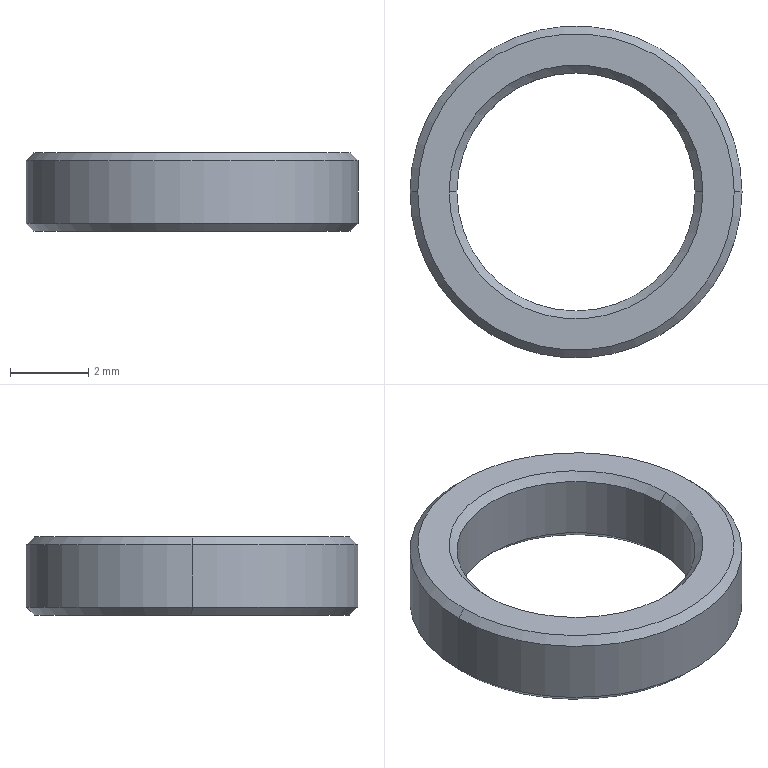Part | NX | features BREP 1 | 1 solid | 14 faces | box 8.5 x 8.5 x 2 mm | volume 53.206 mm3 | cone 8 | cylinder 4 | plane 2 | commonest cylinder face diameters 6.1 x2 8.5 x2
STEP:
#1=CARTESIAN_POINT('',(-3.25,0.,2.));
#2=VERTEX_POINT('',#1);
#3=CARTESIAN_POINT('',(-3.05,0.,1.8));
#4=VERTEX_POINT('',#3);
#5=CARTESIAN_POINT('',(-3.05,0.,1.8));
#6=DIRECTION('',(-0.7071,0.,0.7071));
#7=VECTOR('',#6,1000.);
#8=LINE('',#5,#7);
#9=EDGE_CURVE('',#2,#4,#8,.F.);
#10=ORIENTED_EDGE('',*,*,#9,.T.);
#11=CARTESIAN_POINT('',(3.05,0.,1.8));
#12=VERTEX_POINT('',#11);
#13=CARTESIAN_POINT('',(0.,0.,1.8));
#14=DIRECTION('',(0.,0.,1.));
#15=DIRECTION('',(1.,0.,0.));
#16=AXIS2_PLACEMENT_3D('',#13,#14,#15);
#17=CIRCLE('',#16,3.05);
#18=EDGE_CURVE('',#12,#4,#17,.T.);
#19=ORIENTED_EDGE('',*,*,#18,.F.);
#20=CARTESIAN_POINT('',(3.25,0.,2.));
#21=VERTEX_POINT('',#20);
#22=CARTESIAN_POINT('',(3.05,0.,1.8));
#23=DIRECTION('',(0.7071,0.,0.7071));
#24=VECTOR('',#23,1000.);
#25=LINE('',#22,#24);
#26=EDGE_CURVE('',#21,#12,#25,.F.);
#27=ORIENTED_EDGE('',*,*,#26,.F.);
#28=CARTESIAN_POINT('',(0.,0.,2.));
#29=DIRECTION('',(0.,0.,-1.));
#30=DIRECTION('',(1.,0.,0.));
#31=AXIS2_PLACEMENT_3D('',#28,#29,#30);
#32=CIRCLE('',#31,3.25);
#33=EDGE_CURVE('',#2,#21,#32,.T.);
#34=ORIENTED_EDGE('',*,*,#33,.F.);
#35=EDGE_LOOP('',(#10,#19,#27,#34));
#36=FACE_BOUND('',#35,.T.);
#37=CARTESIAN_POINT('',(0.,0.,1.8));
#38=DIRECTION('',(0.,0.,1.));
#39=DIRECTION('',(1.,0.,0.));
#40=AXIS2_PLACEMENT_3D('',#37,#38,#39);
#41=CONICAL_SURFACE('',#40,3.05,0.7854);
#42=ADVANCED_FACE('',(#36),#41,.F.);
#43=CARTESIAN_POINT('',(4.05,0.,2.));
#44=VERTEX_POINT('',#43);
#45=CARTESIAN_POINT('',(4.25,0.,1.8));
#46=VERTEX_POINT('',#45);
#47=CARTESIAN_POINT('',(4.05,0.,2.));
#48=DIRECTION('',(0.7071,0.,-0.7071));
#49=VECTOR('',#48,1000.);
#50=LINE('',#47,#49);
#51=EDGE_CURVE('',#44,#46,#50,.T.);
#52=ORIENTED_EDGE('',*,*,#51,.F.);
#53=CARTESIAN_POINT('',(-4.05,0.,2.));
#54=VERTEX_POINT('',#53);
#55=CARTESIAN_POINT('',(0.,0.,2.));
#56=DIRECTION('',(0.,0.,1.));
#57=DIRECTION('',(1.,0.,0.));
#58=AXIS2_PLACEMENT_3D('',#55,#56,#57);
#59=CIRCLE('',#58,4.05);
#60=EDGE_CURVE('',#54,#44,#59,.T.);
#61=ORIENTED_EDGE('',*,*,#60,.F.);
#62=CARTESIAN_POINT('',(-4.25,0.,1.8));
#63=VERTEX_POINT('',#62);
#64=CARTESIAN_POINT('',(-4.05,0.,2.));
#65=DIRECTION('',(-0.7071,0.,-0.7071));
#66=VECTOR('',#65,1000.);
#67=LINE('',#64,#66);
#68=EDGE_CURVE('',#54,#63,#67,.T.);
#69=ORIENTED_EDGE('',*,*,#68,.T.);
#70=CARTESIAN_POINT('',(0.,0.,1.8));
#71=DIRECTION('',(0.,0.,-1.));
#72=DIRECTION('',(1.,0.,0.));
#73=AXIS2_PLACEMENT_3D('',#70,#71,#72);
#74=CIRCLE('',#73,4.25);
#75=EDGE_CURVE('',#46,#63,#74,.T.);
#76=ORIENTED_EDGE('',*,*,#75,.F.);
#77=EDGE_LOOP('',(#52,#61,#69,#76));
#78=FACE_BOUND('',#77,.T.);
#79=CARTESIAN_POINT('',(0.,0.,2.));
#80=DIRECTION('',(0.,0.,-1.));
#81=DIRECTION('',(-1.,0.,0.));
#82=AXIS2_PLACEMENT_3D('',#79,#80,#81);
#83=CONICAL_SURFACE('',#82,4.05,0.7854);
#84=ADVANCED_FACE('',(#78),#83,.T.);
#85=CARTESIAN_POINT('',(3.05,0.,0.2));
#86=VERTEX_POINT('',#85);
#87=CARTESIAN_POINT('',(3.25,0.,0.));
#88=VERTEX_POINT('',#87);
#89=CARTESIAN_POINT('',(3.25,0.,0.));
#90=DIRECTION('',(0.7071,0.,-0.7071));
#91=VECTOR('',#90,1000.);
#92=LINE('',#89,#91);
#93=EDGE_CURVE('',#86,#88,#92,.T.);
#94=ORIENTED_EDGE('',*,*,#93,.F.);
#95=CARTESIAN_POINT('',(-3.05,0.,0.2));
#96=VERTEX_POINT('',#95);
#97=CARTESIAN_POINT('',(0.,0.,0.2));
#98=DIRECTION('',(0.,0.,-1.));
#99=DIRECTION('',(1.,0.,0.));
#100=AXIS2_PLACEMENT_3D('',#97,#98,#99);
#101=CIRCLE('',#100,3.05);
#102=EDGE_CURVE('',#96,#86,#101,.T.);
#103=ORIENTED_EDGE('',*,*,#102,.F.);
#104=CARTESIAN_POINT('',(-3.25,0.,0.));
#105=VERTEX_POINT('',#104);
#106=CARTESIAN_POINT('',(-3.25,0.,0.));
#107=DIRECTION('',(-0.7071,0.,-0.7071));
#108=VECTOR('',#107,1000.);
#109=LINE('',#106,#108);
#110=EDGE_CURVE('',#96,#105,#109,.T.);
#111=ORIENTED_EDGE('',*,*,#110,.T.);
#112=CARTESIAN_POINT('',(0.,0.,0.));
#113=DIRECTION('',(0.,0.,1.));
#114=DIRECTION('',(1.,0.,0.));
#115=AXIS2_PLACEMENT_3D('',#112,#113,#114);
#116=CIRCLE('',#115,3.25);
#117=EDGE_CURVE('',#88,#105,#116,.T.);
#118=ORIENTED_EDGE('',*,*,#117,.F.);
#119=EDGE_LOOP('',(#94,#103,#111,#118));
#120=FACE_BOUND('',#119,.T.);
#121=CARTESIAN_POINT('',(0.,0.,0.));
#122=DIRECTION('',(0.,0.,-1.));
#123=DIRECTION('',(-1.,0.,0.));
#124=AXIS2_PLACEMENT_3D('',#121,#122,#123);
#125=CONICAL_SURFACE('',#124,3.25,0.7854);
#126=ADVANCED_FACE('',(#120),#125,.F.);
#127=CARTESIAN_POINT('',(-4.25,0.,0.2));
#128=VERTEX_POINT('',#127);
#129=CARTESIAN_POINT('',(-4.05,0.,0.));
#130=VERTEX_POINT('',#129);
#131=CARTESIAN_POINT('',(-4.25,0.,0.2));
#132=DIRECTION('',(-0.7071,0.,0.7071));
#133=VECTOR('',#132,1000.);
#134=LINE('',#131,#133);
#135=EDGE_CURVE('',#128,#130,#134,.F.);
#136=ORIENTED_EDGE('',*,*,#135,.T.);
#137=CARTESIAN_POINT('',(4.05,0.,0.));
#138=VERTEX_POINT('',#137);
#139=CARTESIAN_POINT('',(0.,0.,0.));
#140=DIRECTION('',(0.,0.,-1.));
#141=DIRECTION('',(1.,0.,0.));
#142=AXIS2_PLACEMENT_3D('',#139,#140,#141);
#143=CIRCLE('',#142,4.05);
#144=EDGE_CURVE('',#138,#130,#143,.T.);
#145=ORIENTED_EDGE('',*,*,#144,.F.);
#146=CARTESIAN_POINT('',(4.25,0.,0.2));
#147=VERTEX_POINT('',#146);
#148=CARTESIAN_POINT('',(4.25,0.,0.2));
#149=DIRECTION('',(0.7071,0.,0.7071));
#150=VECTOR('',#149,1000.);
#151=LINE('',#148,#150);
#152=EDGE_CURVE('',#147,#138,#151,.F.);
#153=ORIENTED_EDGE('',*,*,#152,.F.);
#154=CARTESIAN_POINT('',(0.,0.,0.2));
#155=DIRECTION('',(0.,0.,1.));
#156=DIRECTION('',(1.,0.,0.));
#157=AXIS2_PLACEMENT_3D('',#154,#155,#156);
#158=CIRCLE('',#157,4.25);
#159=EDGE_CURVE('',#128,#147,#158,.T.);
#160=ORIENTED_EDGE('',*,*,#159,.F.);
#161=EDGE_LOOP('',(#136,#145,#153,#160));
#162=FACE_BOUND('',#161,.T.);
#163=CARTESIAN_POINT('',(0.,0.,0.2));
#164=DIRECTION('',(0.,0.,1.));
#165=DIRECTION('',(1.,0.,0.));
#166=AXIS2_PLACEMENT_3D('',#163,#164,#165);
#167=CONICAL_SURFACE('',#166,4.25,0.7854);
#168=ADVANCED_FACE('',(#162),#167,.T.);
#169=CARTESIAN_POINT('',(3.05,0.,2.));
#170=DIRECTION('',(0.,0.,-1.));
#171=VECTOR('',#170,1000.);
#172=LINE('',#169,#171);
#173=EDGE_CURVE('',#12,#86,#172,.T.);
#174=ORIENTED_EDGE('',*,*,#173,.F.);
#175=ORIENTED_EDGE('',*,*,#18,.T.);
#176=CARTESIAN_POINT('',(-3.05,0.,2.));
#177=DIRECTION('',(0.,0.,-1.));
#178=VECTOR('',#177,1000.);
#179=LINE('',#176,#178);
#180=EDGE_CURVE('',#4,#96,#179,.T.);
#181=ORIENTED_EDGE('',*,*,#180,.T.);
#182=ORIENTED_EDGE('',*,*,#102,.T.);
#183=EDGE_LOOP('',(#174,#175,#181,#182));
#184=FACE_BOUND('',#183,.T.);
#185=CARTESIAN_POINT('',(0.,0.,2.));
#186=DIRECTION('',(0.,0.,-1.));
#187=DIRECTION('',(-1.,0.,0.));
#188=AXIS2_PLACEMENT_3D('',#185,#186,#187);
#189=CYLINDRICAL_SURFACE('',#188,3.05);
#190=ADVANCED_FACE('',(#184),#189,.F.);
#191=CARTESIAN_POINT('',(4.25,0.,2.));
#192=DIRECTION('',(0.,0.,-1.));
#193=VECTOR('',#192,1000.);
#194=LINE('',#191,#193);
#195=EDGE_CURVE('',#46,#147,#194,.T.);
#196=ORIENTED_EDGE('',*,*,#195,.F.);
#197=ORIENTED_EDGE('',*,*,#75,.T.);
#198=CARTESIAN_POINT('',(-4.25,0.,2.));
#199=DIRECTION('',(0.,0.,-1.));
#200=VECTOR('',#199,1000.);
#201=LINE('',#198,#200);
#202=EDGE_CURVE('',#63,#128,#201,.T.);
#203=ORIENTED_EDGE('',*,*,#202,.T.);
#204=ORIENTED_EDGE('',*,*,#159,.T.);
#205=EDGE_LOOP('',(#196,#197,#203,#204));
#206=FACE_BOUND('',#205,.T.);
#207=CARTESIAN_POINT('',(0.,0.,2.));
#208=DIRECTION('',(0.,0.,-1.));
#209=DIRECTION('',(-1.,0.,0.));
#210=AXIS2_PLACEMENT_3D('',#207,#208,#209);
#211=CYLINDRICAL_SURFACE('',#210,4.25);
#212=ADVANCED_FACE('',(#206),#211,.T.);
#213=CARTESIAN_POINT('',(0.,0.,0.));
#214=DIRECTION('',(0.,0.,1.));
#215=DIRECTION('',(1.,0.,0.));
#216=AXIS2_PLACEMENT_3D('',#213,#214,#215);
#217=CIRCLE('',#216,3.25);
#218=EDGE_CURVE('',#105,#88,#217,.T.);
#219=ORIENTED_EDGE('',*,*,#218,.T.);
#220=ORIENTED_EDGE('',*,*,#117,.T.);
#221=EDGE_LOOP('',(#219,#220));
#222=FACE_BOUND('',#221,.T.);
#223=ORIENTED_EDGE('',*,*,#144,.T.);
#224=CARTESIAN_POINT('',(0.,0.,0.));
#225=DIRECTION('',(0.,0.,-1.));
#226=DIRECTION('',(1.,0.,0.));
#227=AXIS2_PLACEMENT_3D('',#224,#225,#226);
#228=CIRCLE('',#227,4.05);
#229=EDGE_CURVE('',#130,#138,#228,.T.);
#230=ORIENTED_EDGE('',*,*,#229,.T.);
#231=EDGE_LOOP('',(#223,#230));
#232=FACE_BOUND('',#231,.T.);
#233=CARTESIAN_POINT('',(0.,0.,0.));
#234=DIRECTION('',(0.,0.,1.));
#235=DIRECTION('',(1.,0.,0.));
#236=AXIS2_PLACEMENT_3D('',#233,#234,#235);
#237=PLANE('',#236);
#238=ADVANCED_FACE('',(#222,#232),#237,.F.);
#239=CARTESIAN_POINT('',(0.,0.,2.));
#240=DIRECTION('',(0.,0.,-1.));
#241=DIRECTION('',(1.,0.,0.));
#242=AXIS2_PLACEMENT_3D('',#239,#240,#241);
#243=CIRCLE('',#242,3.25);
#244=EDGE_CURVE('',#21,#2,#243,.T.);
#245=ORIENTED_EDGE('',*,*,#244,.T.);
#246=ORIENTED_EDGE('',*,*,#33,.T.);
#247=EDGE_LOOP('',(#245,#246));
#248=FACE_BOUND('',#247,.T.);
#249=ORIENTED_EDGE('',*,*,#60,.T.);
#250=CARTESIAN_POINT('',(0.,0.,2.));
#251=DIRECTION('',(0.,0.,1.));
#252=DIRECTION('',(1.,0.,0.));
#253=AXIS2_PLACEMENT_3D('',#250,#251,#252);
#254=CIRCLE('',#253,4.05);
#255=EDGE_CURVE('',#44,#54,#254,.T.);
#256=ORIENTED_EDGE('',*,*,#255,.T.);
#257=EDGE_LOOP('',(#249,#256));
#258=FACE_BOUND('',#257,.T.);
#259=CARTESIAN_POINT('',(0.,0.,2.));
#260=DIRECTION('',(0.,0.,1.));
#261=DIRECTION('',(1.,0.,0.));
#262=AXIS2_PLACEMENT_3D('',#259,#260,#261);
#263=PLANE('',#262);
#264=ADVANCED_FACE('',(#248,#258),#263,.T.);
#265=CARTESIAN_POINT('',(0.,0.,1.8));
#266=DIRECTION('',(0.,0.,-1.));
#267=DIRECTION('',(1.,0.,0.));
#268=AXIS2_PLACEMENT_3D('',#265,#266,#267);
#269=CIRCLE('',#268,4.25);
#270=EDGE_CURVE('',#63,#46,#269,.T.);
#271=ORIENTED_EDGE('',*,*,#270,.T.);
#272=ORIENTED_EDGE('',*,*,#195,.T.);
#273=CARTESIAN_POINT('',(0.,0.,0.2));
#274=DIRECTION('',(0.,0.,1.));
#275=DIRECTION('',(1.,0.,0.));
#276=AXIS2_PLACEMENT_3D('',#273,#274,#275);
#277=CIRCLE('',#276,4.25);
#278=EDGE_CURVE('',#147,#128,#277,.T.);
#279=ORIENTED_EDGE('',*,*,#278,.T.);
#280=ORIENTED_EDGE('',*,*,#202,.F.);
#281=EDGE_LOOP('',(#271,#272,#279,#280));
#282=FACE_BOUND('',#281,.T.);
#283=CARTESIAN_POINT('',(0.,0.,2.));
#284=DIRECTION('',(0.,0.,-1.));
#285=DIRECTION('',(-1.,0.,0.));
#286=AXIS2_PLACEMENT_3D('',#283,#284,#285);
#287=CYLINDRICAL_SURFACE('',#286,4.25);
#288=ADVANCED_FACE('',(#282),#287,.T.);
#289=CARTESIAN_POINT('',(0.,0.,1.8));
#290=DIRECTION('',(0.,0.,1.));
#291=DIRECTION('',(1.,0.,0.));
#292=AXIS2_PLACEMENT_3D('',#289,#290,#291);
#293=CIRCLE('',#292,3.05);
#294=EDGE_CURVE('',#4,#12,#293,.T.);
#295=ORIENTED_EDGE('',*,*,#294,.T.);
#296=ORIENTED_EDGE('',*,*,#173,.T.);
#297=CARTESIAN_POINT('',(0.,0.,0.2));
#298=DIRECTION('',(0.,0.,-1.));
#299=DIRECTION('',(1.,0.,0.));
#300=AXIS2_PLACEMENT_3D('',#297,#298,#299);
#301=CIRCLE('',#300,3.05);
#302=EDGE_CURVE('',#86,#96,#301,.T.);
#303=ORIENTED_EDGE('',*,*,#302,.T.);
#304=ORIENTED_EDGE('',*,*,#180,.F.);
#305=EDGE_LOOP('',(#295,#296,#303,#304));
#306=FACE_BOUND('',#305,.T.);
#307=CARTESIAN_POINT('',(0.,0.,2.));
#308=DIRECTION('',(0.,0.,-1.));
#309=DIRECTION('',(-1.,0.,0.));
#310=AXIS2_PLACEMENT_3D('',#307,#308,#309);
#311=CYLINDRICAL_SURFACE('',#310,3.05);
#312=ADVANCED_FACE('',(#306),#311,.F.);
#313=ORIENTED_EDGE('',*,*,#229,.F.);
#314=ORIENTED_EDGE('',*,*,#135,.F.);
#315=ORIENTED_EDGE('',*,*,#278,.F.);
#316=ORIENTED_EDGE('',*,*,#152,.T.);
#317=EDGE_LOOP('',(#313,#314,#315,#316));
#318=FACE_BOUND('',#317,.T.);
#319=CARTESIAN_POINT('',(0.,0.,0.2));
#320=DIRECTION('',(0.,0.,1.));
#321=DIRECTION('',(1.,0.,0.));
#322=AXIS2_PLACEMENT_3D('',#319,#320,#321);
#323=CONICAL_SURFACE('',#322,4.25,0.7854);
#324=ADVANCED_FACE('',(#318),#323,.T.);
#325=ORIENTED_EDGE('',*,*,#302,.F.);
#326=ORIENTED_EDGE('',*,*,#93,.T.);
#327=ORIENTED_EDGE('',*,*,#218,.F.);
#328=ORIENTED_EDGE('',*,*,#110,.F.);
#329=EDGE_LOOP('',(#325,#326,#327,#328));
#330=FACE_BOUND('',#329,.T.);
#331=CARTESIAN_POINT('',(0.,0.,0.));
#332=DIRECTION('',(0.,0.,-1.));
#333=DIRECTION('',(-1.,0.,0.));
#334=AXIS2_PLACEMENT_3D('',#331,#332,#333);
#335=CONICAL_SURFACE('',#334,3.25,0.7854);
#336=ADVANCED_FACE('',(#330),#335,.F.);
#337=ORIENTED_EDGE('',*,*,#255,.F.);
#338=ORIENTED_EDGE('',*,*,#51,.T.);
#339=ORIENTED_EDGE('',*,*,#270,.F.);
#340=ORIENTED_EDGE('',*,*,#68,.F.);
#341=EDGE_LOOP('',(#337,#338,#339,#340));
#342=FACE_BOUND('',#341,.T.);
#343=CARTESIAN_POINT('',(0.,0.,2.));
#344=DIRECTION('',(0.,0.,-1.));
#345=DIRECTION('',(-1.,0.,0.));
#346=AXIS2_PLACEMENT_3D('',#343,#344,#345);
#347=CONICAL_SURFACE('',#346,4.05,0.7854);
#348=ADVANCED_FACE('',(#342),#347,.T.);
#349=ORIENTED_EDGE('',*,*,#294,.F.);
#350=ORIENTED_EDGE('',*,*,#9,.F.);
#351=ORIENTED_EDGE('',*,*,#244,.F.);
#352=ORIENTED_EDGE('',*,*,#26,.T.);
#353=EDGE_LOOP('',(#349,#350,#351,#352));
#354=FACE_BOUND('',#353,.T.);
#355=CARTESIAN_POINT('',(0.,0.,1.8));
#356=DIRECTION('',(0.,0.,1.));
#357=DIRECTION('',(1.,0.,0.));
#358=AXIS2_PLACEMENT_3D('',#355,#356,#357);
#359=CONICAL_SURFACE('',#358,3.05,0.7854);
#360=ADVANCED_FACE('',(#354),#359,.F.);
#361=CLOSED_SHELL('',(#42,#84,#126,#168,#190,#212,#238,#264,#288,#312,#324,#336,#348,#360));
#362=MANIFOLD_SOLID_BREP('',#361);
#363=(LENGTH_UNIT()NAMED_UNIT(*)SI_UNIT(.MILLI.,.METRE.));
#364=UNCERTAINTY_MEASURE_WITH_UNIT(LENGTH_MEASURE(0.00001),#363,'','');
#365=(NAMED_UNIT(*)PLANE_ANGLE_UNIT()SI_UNIT($,.RADIAN.));
#366=(NAMED_UNIT(*)SI_UNIT($,.STERADIAN.)SOLID_ANGLE_UNIT());
#367=(GEOMETRIC_REPRESENTATION_CONTEXT(3)GLOBAL_UNCERTAINTY_ASSIGNED_CONTEXT((#364))GLOBAL_UNIT_ASSIGNED_CONTEXT((#363,#365,#366))REPRESENTATION_CONTEXT('',''));
#368=ADVANCED_BREP_SHAPE_REPRESENTATION('',(#362),#367);